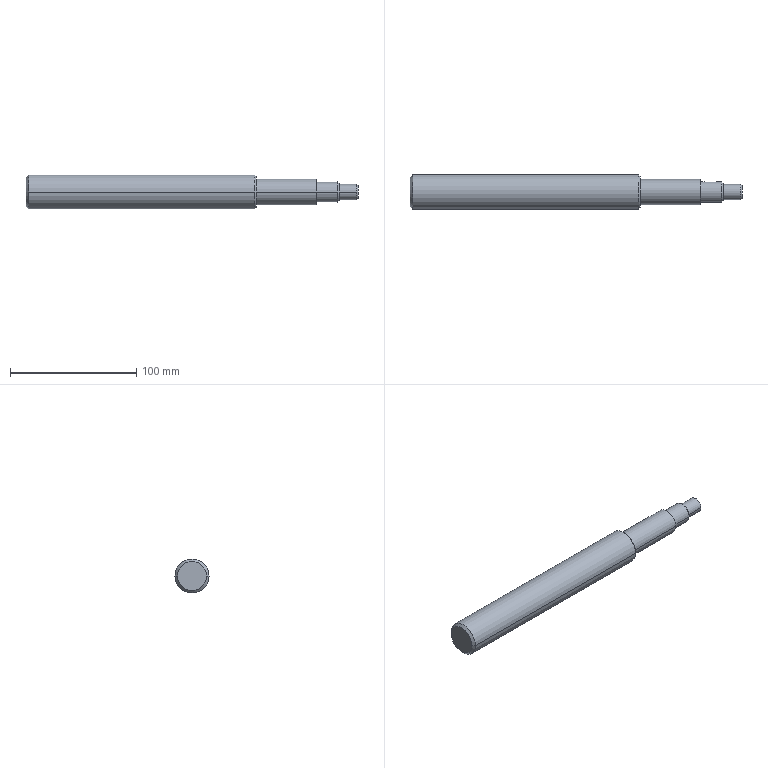Part | STEP file | 1 solid | 28 faces | box 263 x 27 x 27 mm | volume 124305 mm3 | cylinder 12 | cone 8 | plane 8 | commonest cylinder face diameters 5 x4 12 x2 16 x2 20 x2 27 x2